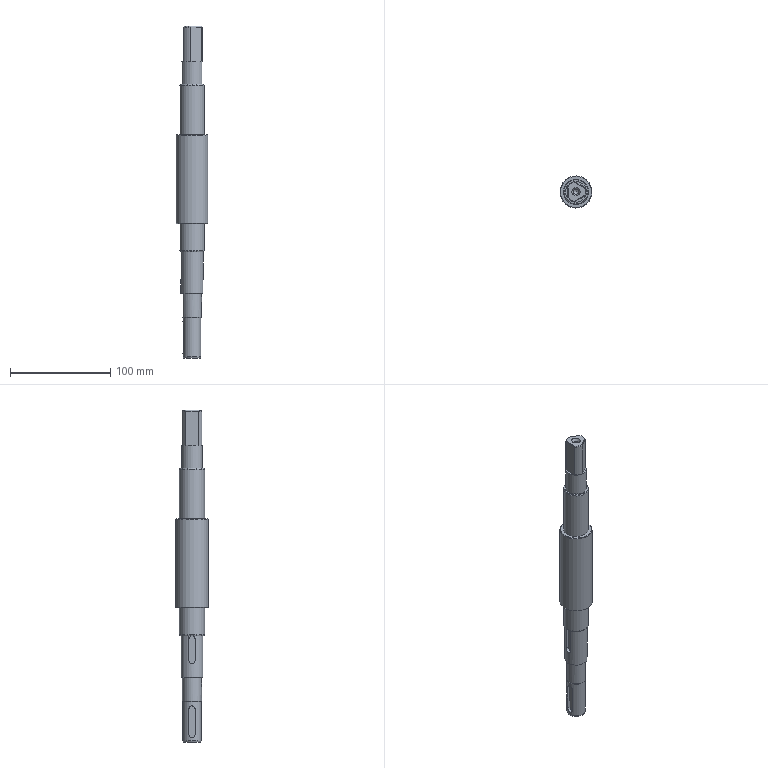NC program | NX | posted with a generic post | part box 32 x 32 x 331.3 mm
Whole program:
N10 G17 G21 G94 G90
(刀补6 , TOOL : D4)
N12 T04 M6
N14 G54
N16 G17 G0 G90 X69.382 Y0.933 B0. C0. S6685 M3
N18 G43 Z30. H4
N20 Z-2.94
N22 G94 G1 X62.644 Z-3.293 F1000.
N24 X62.507 Y0.932 Z-3.3
N26 X62.223 Y0.84 Z-3.316
N28 X61.982 Y0.664 Z-3.331
N30 X61.808 Y0.422 Z-3.347
N32 X61.718 Y0.137 Z-3.363
N34 Y-0.137 Z-3.377
N36 X61.808 Y-0.422 Z-3.393
N38 X61.982 Y-0.664 Z-3.408
N40 X62.223 Y-0.84 Z-3.424
N42 X62.507 Y-0.932 Z-3.44
N44 X62.646 Y-0.933 Z-3.447
N46 X73.552 Z-4.018
N48 G41 X73.65 Y-0.95 D4
N50 X84.656 F1650.
N52 G3 X85.599 Y0. R0.95
N54 X84.656 Y0.95 R0.95
N56 G1 X62.644
N58 G3 X61.701 Y0. R0.95
N60 X62.644 Y-0.95 R0.95
N62 G1 X73.65
N64 X78.154 Z-4.097
N66 X84.656
N68 G3 X85.599 Y0. R0.95
N70 X84.656 Y0.95 R0.95
N72 G1 X62.644
N74 G3 X61.701 Y0. R0.95
N76 X62.644 Y-0.95 R0.95
N78 G1 X73.65
N80 X78.154 Z-4.176
N82 X84.656
N84 G3 X85.599 Y0. R0.95
N86 X84.656 Y0.95 R0.95
N88 G1 X62.644
N90 G3 X61.701 Y0. R0.95
N92 X62.644 Y-0.95 R0.95
N94 G1 X73.65
N96 X78.154 Z-4.254
N98 X84.656
N100 G3 X85.599 Y0. R0.95
N102 X84.656 Y0.95 R0.95
N104 G1 X62.644
N106 G3 X61.701 Y0. R0.95
N108 X62.644 Y-0.95 R0.95
N110 G1 X73.65
N112 X78.154 Z-4.333
N114 X84.656
N116 G3 X85.599 Y0. R0.95
N118 X84.656 Y0.95 R0.95
N120 G1 X62.644
N122 G3 X61.701 Y0. R0.95
N124 X62.644 Y-0.95 R0.95
N126 G1 X73.65
N128 X78.154 Z-4.412
N130 X84.656
N132 G3 X85.599 Y0. R0.95
N134 X84.656 Y0.95 R0.95
N136 G1 X62.644
N138 G3 X61.701 Y0. R0.95
N140 X62.644 Y-0.95 R0.95
N142 G1 X73.65
N144 X78.154 Z-4.49
N146 X84.656
N148 G3 X85.599 Y0. R0.95
N150 X84.656 Y0.95 R0.95
N152 G1 X62.644
N154 G3 X61.701 Y0. R0.95
N156 X62.644 Y-0.95 R0.95
N158 G1 X73.65
N160 X78.154 Z-4.569
N162 X84.656
N164 G3 X85.599 Y0. R0.95
N166 X84.656 Y0.95 R0.95
N168 G1 X62.644
N170 G3 X61.701 Y0. R0.95
N172 X62.644 Y-0.95 R0.95
N174 G1 X73.65
N176 X78.154 Z-4.647
N178 X84.656
N180 G3 X85.599 Y0. R0.95
N182 X84.656 Y0.95 R0.95
N184 G1 X62.644
N186 G3 X61.701 Y0. R0.95
N188 X62.644 Y-0.95 R0.95
N190 G1 X73.65
N192 X78.154 Z-4.726
N194 X84.656
N196 G3 X85.599 Y0. R0.95
N198 X84.656 Y0.95 R0.95
N200 G1 X62.644
N202 G3 X61.701 Y0. R0.95
N204 X62.644 Y-0.95 R0.95
N206 G1 X73.65
N208 X78.154 Z-4.805
N210 X84.656
N212 G3 X85.599 Y0. R0.95
N214 X84.656 Y0.95 R0.95
N216 G1 X62.644
N218 G3 X61.701 Y0. R0.95
N220 X62.644 Y-0.95 R0.95
N222 G1 X73.65
N224 X78.154 Z-4.883
N226 X84.656
N228 G3 X85.599 Y0. R0.95
N230 X84.656 Y0.95 R0.95
N232 G1 X62.644
N234 G3 X61.701 Y0. R0.95
N236 X62.644 Y-0.95 R0.95
N238 G1 X73.65
N240 X78.154 Z-4.962
N242 X84.656
N244 G3 X85.599 Y0. R0.95
N246 X84.656 Y0.95 R0.95
N248 G1 X62.644
N250 G3 X61.701 Y0. R0.95
N252 X62.644 Y-0.95 R0.95
N254 G1 X73.65
N256 X78.154 Z-5.041
N258 X84.65
N260 G3 X85.6 Y0. R0.95
N262 X84.65 Y0.95 R0.95
N264 G1 X62.65
N266 G3 X61.7 Y0. R0.95
N268 X62.65 Y-0.95 R0.95
N270 G1 X73.65
N272 X78.154 Z-5.119
N274 X84.65
N276 G3 X85.6 Y0. R0.95
N278 X84.65 Y0.95 R0.95
N280 G1 X62.65
N282 G3 X61.7 Y0. R0.95
N284 X62.65 Y-0.95 R0.95
N286 G1 X73.65
N288 X78.154 Z-5.198
N290 X84.65
N292 G3 X85.6 Y0. R0.95
N294 X84.65 Y0.95 R0.95
N296 G1 X62.65
N298 G3 X61.7 Y0. R0.95
N300 X62.65 Y-0.95 R0.95
N302 G1 X73.65
N304 X78.154 Z-5.276
N306 X84.65
N308 G3 X85.6 Y0. R0.95
N310 X84.65 Y0.95 R0.95
N312 G1 X62.65
N314 G3 X61.7 Y0. R0.95
N316 X62.65 Y-0.95 R0.95
N318 G1 X73.65
N320 X78.154 Z-5.355
N322 X84.65
N324 G3 X85.6 Y0. R0.95
N326 X84.65 Y0.95 R0.95
N328 G1 X62.65
N330 G3 X61.7 Y0. R0.95
N332 X62.65 Y-0.95 R0.95
N334 G1 X73.65
N336 X78.154 Z-5.434
N338 X84.65
N340 G3 X85.6 Y0. R0.95
N342 X84.65 Y0.95 R0.95
N344 G1 X62.65
N346 G3 X61.7 Y0. R0.95
N348 X62.65 Y-0.95 R0.95
N350 G1 X73.65
N352 X78.154 Z-5.512
N354 X84.65
N356 G3 X85.6 Y0. R0.95
N358 X84.65 Y0.95 R0.95
N360 G1 X62.65
N362 G3 X61.7 Y0. R0.95
N364 X62.65 Y-0.95 R0.95
N366 G1 X73.65
N368 X78.154 Z-5.591
N370 X84.65
N372 G3 X85.6 Y0. R0.95
N374 X84.65 Y0.95 R0.95
N376 G1 X62.65
N378 G3 X61.7 Y0. R0.95
N380 X62.65 Y-0.95 R0.95
N382 G1 X73.65
N384 X78.154 Z-5.67
N386 X84.65
N388 G3 X85.6 Y0. R0.95
N390 X84.65 Y0.95 R0.95
N392 G1 X62.65
N394 G3 X61.7 Y0. R0.95
N396 X62.65 Y-0.95 R0.95
N398 G1 X73.65
N400 X78.154 Z-5.748
N402 X84.65
N404 G3 X85.6 Y0. R0.95
N406 X84.65 Y0.95 R0.95
N408 G1 X62.65
N410 G3 X61.7 Y0. R0.95
N412 X62.65 Y-0.95 R0.95
N414 G1 X73.65
N416 X78.154 Z-5.827
N418 X84.65
N420 G3 X85.6 Y0. R0.95
N422 X84.65 Y0.95 R0.95
N424 G1 X62.65
N426 G3 X61.7 Y0. R0.95
N428 X62.65 Y-0.95 R0.95
N430 G1 X73.65
N432 X78.154 Z-5.905
N434 X84.65
N436 G3 X85.6 Y0. R0.95
N438 X84.65 Y0.95 R0.95
N440 G1 X62.65
N442 G3 X61.7 Y0. R0.95
N444 X62.65 Y-0.95 R0.95
N446 G1 X73.65
N448 X78.154 Z-5.984
N450 X84.65
N452 G3 X85.6 Y0. R0.95
N454 X84.65 Y0.95 R0.95
N456 G1 X62.65
N458 G3 X61.7 Y0. R0.95
N460 X62.65 Y-0.95 R0.95
N462 G1 X73.65
N464 X78.154 Z-6.063
N466 X84.65
N468 G3 X85.6 Y0. R0.95
N470 X84.65 Y0.95 R0.95
N472 G1 X62.65
N474 G3 X61.7 Y0. R0.95
N476 X62.65 Y-0.95 R0.95
N478 G1 X73.65
N480 X78.154 Z-6.141
N482 X84.65
N484 G3 X85.6 Y0. R0.95
N486 X84.65 Y0.95 R0.95
N488 G1 X62.65
N490 G3 X61.7 Y0. R0.95
N492 X62.65 Y-0.95 R0.95
N494 G1 X73.65
N496 X78.154 Z-6.22
N498 X84.65
N500 G3 X85.6 Y0. R0.95
N502 X84.65 Y0.95 R0.95
N504 G1 X62.65
N506 G3 X61.7 Y0. R0.95
N508 X62.65 Y-0.95 R0.95
N510 G1 X73.65
N512 X78.154 Z-6.299
N514 X84.65
N516 G3 X85.6 Y0. R0.95
N518 X84.65 Y0.95 R0.95
N520 G1 X62.65
N522 G3 X61.7 Y0. R0.95
N524 X62.65 Y-0.95 R0.95
N526 G1 X73.65
N528 X78.154 Z-6.377
N530 X84.65
N532 G3 X85.6 Y0. R0.95
N534 X84.65 Y0.95 R0.95
N536 G1 X62.65
N538 G3 X61.7 Y0. R0.95
N540 X62.65 Y-0.95 R0.95
N542 G1 X73.65
N544 X78.154 Z-6.456
N546 X84.65
N548 G3 X85.6 Y0. R0.95
N550 X84.65 Y0.95 R0.95
N552 G1 X62.65
N554 G3 X61.7 Y0. R0.95
N556 X62.65 Y-0.95 R0.95
N558 G1 X73.65
N560 X78.154 Z-6.534
N562 X84.65
N564 G3 X85.6 Y0. R0.95
N566 X84.65 Y0.95 R0.95
N568 G1 X62.65
N570 G3 X61.7 Y0. R0.95
N572 X62.65 Y-0.95 R0.95
N574 G1 X73.65
N576 X78.154 Z-6.613
N578 X84.65
N580 G3 X85.6 Y0. R0.95
N582 X84.65 Y0.95 R0.95
N584 G1 X62.65
N586 G3 X61.7 Y0. R0.95
N588 X62.65 Y-0.95 R0.95
N590 G1 X73.65
N592 X78.154 Z-6.692
N594 X84.65
N596 G3 X85.6 Y0. R0.95
N598 X84.65 Y0.95 R0.95
N600 G1 X62.65
N602 G3 X61.7 Y0. R0.95
N604 X62.65 Y-0.95 R0.95
N606 G1 X73.65
N608 X78.154 Z-6.77
N610 X84.65
N612 G3 X85.6 Y0. R0.95
N614 X84.65 Y0.95 R0.95
N616 G1 X62.65
N618 G3 X61.7 Y0. R0.95
N620 X62.65 Y-0.95 R0.95
N622 G1 X73.65
N624 X78.154 Z-6.849
N626 X84.65
N628 G3 X85.6 Y0. R0.95
N630 X84.65 Y0.95 R0.95
N632 G1 X62.65
N634 G3 X61.7 Y0. R0.95
N636 X62.65 Y-0.95 R0.95
N638 G1 X73.65
N640 X78.154 Z-6.928
N642 X84.65
N644 G3 X85.6 Y0. R0.95
N646 X84.65 Y0.95 R0.95
N648 G1 X62.65
N650 G3 X61.7 Y0. R0.95
N652 X62.65 Y-0.95 R0.95
N654 G1 X73.65
N656 X78.154 Z-7.006
N658 X84.65
N660 G3 X85.6 Y0. R0.95
N662 X84.65 Y0.95 R0.95
N664 G1 X62.65
N666 G3 X61.7 Y0. R0.95
N668 X62.65 Y-0.95 R0.95
N670 G1 X73.65
N672 X78.154 Z-7.085
N674 X84.65
N676 G3 X85.6 Y0. R0.95
N678 X84.65 Y0.95 R0.95
N680 G1 X62.65
N682 G3 X61.7 Y0. R0.95
N684 X62.65 Y-0.95 R0.95
N686 G1 X73.65
N688 X78.154 Z-7.163
N690 X84.65
N692 G3 X85.6 Y0. R0.95
N694 X84.65 Y0.95 R0.95
N696 G1 X62.65
N698 G3 X61.7 Y0. R0.95
N700 X62.65 Y-0.95 R0.95
N702 G1 X73.65
N704 X78.154 Z-7.242
N706 X84.65
N708 G3 X85.6 Y0. R0.95
N710 X84.65 Y0.95 R0.95
N712 G1 X62.65
N714 G3 X61.7 Y0. R0.95
N716 X62.65 Y-0.95 R0.95
N718 G1 X73.65
N720 X78.154 Z-7.321
N722 X84.65
N724 G3 X85.6 Y0. R0.95
N726 X84.65 Y0.95 R0.95
N728 G1 X62.65
N730 G3 X61.7 Y0. R0.95
N732 X62.65 Y-0.95 R0.95
N734 G1 X73.65
N736 X78.154 Z-7.399
N738 X84.65
N740 G3 X85.6 Y0. R0.95
N742 X84.65 Y0.95 R0.95
N744 G1 X62.65
N746 G3 X61.7 Y0. R0.95
N748 X62.65 Y-0.95 R0.95
N750 G1 X73.65
N752 X78.154 Z-7.478
N754 X84.65
N756 G3 X85.6 Y0. R0.95
N758 X84.65 Y0.95 R0.95
N760 G1 X62.65
N762 G3 X61.7 Y0. R0.95
N764 X62.65 Y-0.95 R0.95
N766 G1 X73.65
N768 X78.154 Z-7.557
N770 X84.65
N772 G3 X85.6 Y0. R0.95
N774 X84.65 Y0.95 R0.95
N776 G1 X62.65
N778 G3 X61.7 Y0. R0.95
N780 X62.65 Y-0.95 R0.95
N782 G1 X73.65
N784 X78.154 Z-7.635
N786 X84.65
N788 G3 X85.6 Y0. R0.95
N790 X84.65 Y0.95 R0.95
N792 G1 X62.65
N794 G3 X61.7 Y0. R0.95
N796 X62.65 Y-0.95 R0.95
N798 G1 X73.65
N800 X78.154 Z-7.714
N802 X84.65
N804 G3 X85.6 Y0. R0.95
N806 X84.65 Y0.95 R0.95
N808 G1 X62.65
N810 G3 X61.7 Y0. R0.95
N812 X62.65 Y-0.95 R0.95
N814 G1 X73.65
N816 X78.154 Z-7.792
N818 X84.65
N820 G3 X85.6 Y0. R0.95
N822 X84.65 Y0.95 R0.95
N824 G1 X62.65
N826 G3 X61.7 Y0. R0.95
N828 X62.65 Y-0.95 R0.95
N830 G1 X73.65
N832 X78.154 Z-7.871
N834 X84.65
N836 G3 X85.6 Y0. R0.95
N838 X84.65 Y0.95 R0.95
N840 G1 X62.65
N842 G3 X61.7 Y0. R0.95
N844 X62.65 Y-0.95 R0.95
N846 G1 X73.65
N848 X78.154 Z-7.95
N850 X84.65
N852 G3 X85.6 Y0. R0.95
N854 X84.65 Y0.95 R0.95
N856 G1 X62.65
N858 G3 X61.7 Y0. R0.95
N860 X62.65 Y-0.95 R0.95
N862 G1 X73.65
N864 X78.154 Z-8.028
N866 X84.65
N868 G3 X85.6 Y0. R0.95
N870 X84.65 Y0.95 R0.95
N872 G1 X62.65
N874 G3 X61.7 Y0. R0.95
N876 X62.65 Y-0.95 R0.95
N878 G1 X73.65
N880 X78.154 Z-8.107
N882 X84.65
N884 G3 X85.6 Y0. R0.95
N886 X84.65 Y0.95 R0.95
N888 G1 X62.65
N890 G3 X61.7 Y0. R0.95
N892 X62.65 Y-0.95 R0.95
N894 G1 X73.65
N896 X78.154 Z-8.186
N898 X84.65
N900 G3 X85.6 Y0. R0.95
N902 X84.65 Y0.95 R0.95
N904 G1 X62.65
N906 G3 X61.7 Y0. R0.95
N908 X62.65 Y-0.95 R0.95
N910 G1 X73.65
N912 X78.154 Z-8.264
N914 X84.65
N916 G3 X85.6 Y0. R0.95
N918 X84.65 Y0.95 R0.95
N920 G1 X62.65
N922 G3 X61.7 Y0. R0.95
N924 X62.65 Y-0.95 R0.95
N926 G1 X73.65
N928 X78.154 Z-8.343
N930 X84.65
N932 G3 X85.6 Y0. R0.95
N934 X84.65 Y0.95 R0.95
N936 G1 X62.65
N938 G3 X61.7 Y0. R0.95
N940 X62.65 Y-0.95 R0.95
N942 G1 X73.65
N944 X78.154 Z-8.421
N946 X84.65
N948 G3 X85.6 Y0. R0.95
N950 X84.65 Y0.95 R0.95
N952 G1 X62.65
N954 G3 X61.7 Y0. R0.95
N956 X62.65 Y-0.95 R0.95
N958 G1 X73.65
N960 X78.154 Z-8.5
N962 X84.65
N964 G3 X85.6 Y0. R0.95
N966 X84.65 Y0.95 R0.95
N968 G1 X62.65
N970 G3 X61.7 Y0. R0.95
N972 X62.65 Y-0.95 R0.95
N974 G1 X78.154
N976 G40
N978 X78.253 Y-0.933
N980 Z-7.5
N982 G0 Z30.
(刀补6_COPY , TOOL : D4)
N984 X137.381 Y0.933
N986 Z-5.884
N988 G1 X132.644 Z-6.133 F1000.
N990 X132.507 Y0.932 Z-6.14
N992 X132.223 Y0.84 Z-6.156
N994 X131.982 Y0.664 Z-6.171
N996 X131.808 Y0.422 Z-6.187
N998 X131.718 Y0.137 Z-6.203
N1000 Y-0.137 Z-6.217
N1002 X131.808 Y-0.422 Z-6.233
N1004 X131.982 Y-0.664 Z-6.248
N1006 X132.223 Y-0.84 Z-6.264
N1008 X132.507 Y-0.932 Z-6.279
N1010 X132.646 Y-0.933 Z-6.287
N1012 X145.552 Z-6.963
N1014 G41 X145.65 Y-0.95
N1016 X158.656 F1650.
N1018 G3 X159.599 Y0. R0.95
N1020 X158.656 Y0.95 R0.95
N1022 G1 X132.644
N1024 G3 X131.701 Y0. R0.95
N1026 X132.644 Y-0.95 R0.95
N1028 G1 X145.65
N1030 X150.153 Z-7.042
N1032 X158.65
N1034 G3 X159.6 Y0. R0.95
N1036 X158.65 Y0.95 R0.95
N1038 G1 X132.65
N1040 G3 X131.7 Y0. R0.95
N1042 X132.65 Y-0.95 R0.95
N1044 G1 X145.65
N1046 X150.153 Z-7.12
N1048 X158.65
N1050 G3 X159.6 Y0. R0.95
N1052 X158.65 Y0.95 R0.95
N1054 G1 X132.65
N1056 G3 X131.7 Y0. R0.95
N1058 X132.65 Y-0.95 R0.95
N1060 G1 X145.65
N1062 X150.153 Z-7.199
N1064 X158.65
N1066 G3 X159.6 Y0. R0.95
N1068 X158.65 Y0.95 R0.95
N1070 G1 X132.65
N1072 G3 X131.7 Y0. R0.95
N1074 X132.65 Y-0.95 R0.95
N1076 G1 X145.65
N1078 X150.153 Z-7.277
N1080 X158.65
N1082 G3 X159.6 Y0. R0.95
N1084 X158.65 Y0.95 R0.95
N1086 G1 X132.65
N1088 G3 X131.7 Y0. R0.95
N1090 X132.65 Y-0.95 R0.95
N1092 G1 X145.65
N1094 X150.153 Z-7.356
N1096 X158.65
N1098 G3 X159.6 Y0. R0.95
N1100 X158.65 Y0.95 R0.95
N1102 G1 X132.65
N1104 G3 X131.7 Y0. R0.95
N1106 X132.65 Y-0.95 R0.95
N1108 G1 X145.65
N1110 X150.153 Z-7.435
N1112 X158.65
N1114 G3 X159.6 Y0. R0.95
N1116 X158.65 Y0.95 R0.95
N1118 G1 X132.65
N1120 G3 X131.7 Y0. R0.95
N1122 X132.65 Y-0.95 R0.95
N1124 G1 X145.65
N1126 X150.153 Z-7.513
N1128 X158.65
N1130 G3 X159.6 Y0. R0.95
N1132 X158.65 Y0.95 R0.95
N1134 G1 X132.65
N1136 G3 X131.7 Y0. R0.95
N1138 X132.65 Y-0.95 R0.95
N1140 G1 X145.65
N1142 X150.153 Z-7.592
N1144 X158.65
N1146 G3 X159.6 Y0. R0.95
N1148 X158.65 Y0.95 R0.95
N1150 G1 X132.65
N1152 G3 X131.7 Y0. R0.95
N1154 X132.65 Y-0.95 R0.95
N1156 G1 X145.65
N1158 X150.153 Z-7.67
N1160 X158.65
N1162 G3 X159.6 Y0. R0.95
N1164 X158.65 Y0.95 R0.95
N1166 G1 X132.65
N1168 G3 X131.7 Y0. R0.95
N1170 X132.65 Y-0.95 R0.95
N1172 G1 X145.65
N1174 X150.153 Z-7.749
N1176 X158.65
N1178 G3 X159.6 Y0. R0.95
N1180 X158.65 Y0.95 R0.95
N1182 G1 X132.65
N1184 G3 X131.7 Y0. R0.95
N1186 X132.65 Y-0.95 R0.95
N1188 G1 X145.65
N1190 X150.153 Z-7.828
N1192 X158.65
N1194 G3 X159.6 Y0. R0.95
N1196 X158.65 Y0.95 R0.95
N1198 G1 X132.65
N1200 G3 X131.7 Y0. R0.95
N1202 X132.65 Y-0.95 R0.95
N1204 G1 X145.65
N1206 X150.153 Z-7.906
N1208 X158.65
N1210 G3 X159.6 Y0. R0.95
N1212 X158.65 Y0.95 R0.95
N1214 G1 X132.65
N1216 G3 X131.7 Y0. R0.95
N1218 X132.65 Y-0.95 R0.95
N1220 G1 X145.65
N1222 X150.153 Z-7.985
N1224 X158.65
N1226 G3 X159.6 Y0. R0.95
N1228 X158.65 Y0.95 R0.95
N1230 G1 X132.65
N1232 G3 X131.7 Y0. R0.95
N1234 X132.65 Y-0.95 R0.95
N1236 G1 X145.65
N1238 X150.153 Z-8.063
N1240 X158.65
N1242 G3 X159.6 Y0. R0.95
N1244 X158.65 Y0.95 R0.95
N1246 G1 X132.65
N1248 G3 X131.7 Y0. R0.95
N1250 X132.65 Y-0.95 R0.95
N1252 G1 X145.65
N1254 X150.153 Z-8.142
N1256 X158.65
N1258 G3 X159.6 Y0. R0.95
N1260 X158.65 Y0.95 R0.95
N1262 G1 X132.65
N1264 G3 X131.7 Y0. R0.95
N1266 X132.65 Y-0.95 R0.95
N1268 G1 X145.65
N1270 X150.153 Z-8.221
N1272 X158.65
N1274 G3 X159.6 Y0. R0.95
N1276 X158.65 Y0.95 R0.95
N1278 G1 X132.65
N1280 G3 X131.7 Y0. R0.95
N1282 X132.65 Y-0.95 R0.95
N1284 G1 X145.65
N1286 X150.153 Z-8.299
N1288 X158.65
N1290 G3 X159.6 Y0. R0.95
N1292 X158.65 Y0.95 R0.95
N1294 G1 X132.65
N1296 G3 X131.7 Y0. R0.95
N1298 X132.65 Y-0.95 R0.95
N1300 G1 X145.65
N1302 X150.153 Z-8.378
N1304 X158.65
N1306 G3 X159.6 Y0. R0.95
N1308 X158.65 Y0.95 R0.95
N1310 G1 X132.65
N1312 G3 X131.7 Y0. R0.95
N1314 X132.65 Y-0.95 R0.95
N1316 G1 X145.65
N1318 X150.153 Z-8.456
N1320 X158.65
N1322 G3 X159.6 Y0. R0.95
N1324 X158.65 Y0.95 R0.95
N1326 G1 X132.65
N1328 G3 X131.7 Y0. R0.95
N1330 X132.65 Y-0.95 R0.95
N1332 G1 X145.65
N1334 X150.153 Z-8.535
N1336 X158.65
N1338 G3 X159.6 Y0. R0.95
N1340 X158.65 Y0.95 R0.95
N1342 G1 X132.65
N1344 G3 X131.7 Y0. R0.95
N1346 X132.65 Y-0.95 R0.95
N1348 G1 X145.65
N1350 X150.153 Z-8.614
N1352 X158.65
N1354 G3 X159.6 Y0. R0.95
N1356 X158.65 Y0.95 R0.95
N1358 G1 X132.65
N1360 G3 X131.7 Y0. R0.95
N1362 X132.65 Y-0.95 R0.95
N1364 G1 X145.65
N1366 X150.153 Z-8.692
N1368 X158.65
N1370 G3 X159.6 Y0. R0.95
N1372 X158.65 Y0.95 R0.95
N1374 G1 X132.65
N1376 G3 X131.7 Y0. R0.95
N1378 X132.65 Y-0.95 R0.95
N1380 G1 X145.65
N1382 X150.153 Z-8.771
N1384 X158.65
N1386 G3 X159.6 Y0. R0.95
N1388 X158.65 Y0.95 R0.95
N1390 G1 X132.65
N1392 G3 X131.7 Y0. R0.95
N1394 X132.65 Y-0.95 R0.95
N1396 G1 X145.65
N1398 X150.153 Z-8.849
N1400 X158.65
N1402 G3 X159.6 Y0. R0.95
N1404 X158.65 Y0.95 R0.95
N1406 G1 X132.65
N1408 G3 X131.7 Y0. R0.95
N1410 X132.65 Y-0.95 R0.95
N1412 G1 X145.65
N1414 X150.153 Z-8.928
N1416 X158.65
N1418 G3 X159.6 Y0. R0.95
N1420 X158.65 Y0.95 R0.95
N1422 G1 X132.65
N1424 G3 X131.7 Y0. R0.95
N1426 X132.65 Y-0.95 R0.95
N1428 G1 X145.65
N1430 X150.153 Z-9.007
N1432 X158.65
N1434 G3 X159.6 Y0. R0.95
N1436 X158.65 Y0.95 R0.95
N1438 G1 X132.65
N1440 G3 X131.7 Y0. R0.95
N1442 X132.65 Y-0.95 R0.95
N1444 G1 X145.65
N1446 X150.153 Z-9.085
N1448 X158.65
N1450 G3 X159.6 Y0. R0.95
N1452 X158.65 Y0.95 R0.95
N1454 G1 X132.65
N1456 G3 X131.7 Y0. R0.95
N1458 X132.65 Y-0.95 R0.95
N1460 G1 X145.65
N1462 X150.153 Z-9.164
N1464 X158.65
N1466 G3 X159.6 Y0. R0.95
N1468 X158.65 Y0.95 R0.95
N1470 G1 X132.65
N1472 G3 X131.7 Y0. R0.95
N1474 X132.65 Y-0.95 R0.95
N1476 G1 X145.65
N1478 X150.153 Z-9.242
N1480 X158.65
N1482 G3 X159.6 Y0. R0.95
N1484 X158.65 Y0.95 R0.95
N1486 G1 X132.65
N1488 G3 X131.7 Y0. R0.95
N1490 X132.65 Y-0.95 R0.95
N1492 G1 X145.65
N1494 X150.153 Z-9.321
N1496 X158.65
N1498 G3 X159.6 Y0. R0.95
N1500 X158.65 Y0.95 R0.95
N1502 G1 X132.65
N1504 G3 X131.7 Y0. R0.95
N1506 X132.65 Y-0.95 R0.95
N1508 G1 X145.65
N1510 X150.153 Z-9.4
N1512 X158.65
N1514 G3 X159.6 Y0. R0.95
N1516 X158.65 Y0.95 R0.95
N1518 G1 X132.65
N1520 G3 X131.7 Y0. R0.95
N1522 X132.65 Y-0.95 R0.95
N1524 G1 X145.65
N1526 X150.153 Z-9.478
N1528 X158.65
N1530 G3 X159.6 Y0. R0.95
N1532 X158.65 Y0.95 R0.95
N1534 G1 X132.65
N1536 G3 X131.7 Y0. R0.95
N1538 X132.65 Y-0.95 R0.95
N1540 G1 X145.65
N1542 X150.153 Z-9.557
N1544 X158.65
N1546 G3 X159.6 Y0. R0.95
N1548 X158.65 Y0.95 R0.95
N1550 G1 X132.65
N1552 G3 X131.7 Y0. R0.95
N1554 X132.65 Y-0.95 R0.95
N1556 G1 X145.65
N1558 X150.153 Z-9.635
N1560 X158.65
N1562 G3 X159.6 Y0. R0.95
N1564 X158.65 Y0.95 R0.95
N1566 G1 X132.65
N1568 G3 X131.7 Y0. R0.95
N1570 X132.65 Y-0.95 R0.95
N1572 G1 X145.65
N1574 X150.153 Z-9.714
N1576 X158.65
N1578 G3 X159.6 Y0. R0.95
N1580 X158.65 Y0.95 R0.95
N1582 G1 X132.65
N1584 G3 X131.7 Y0. R0.95
N1586 X132.65 Y-0.95 R0.95
N1588 G1 X145.65
N1590 X150.153 Z-9.793
N1592 X158.65
N1594 G3 X159.6 Y0. R0.95
N1596 X158.65 Y0.95 R0.95
N1598 G1 X132.65
N1600 G3 X131.7 Y0. R0.95
N1602 X132.65 Y-0.95 R0.95
N1604 G1 X145.65
N1606 X150.153 Z-9.871
N1608 X158.65
N1610 G3 X159.6 Y0. R0.95
N1612 X158.65 Y0.95 R0.95
N1614 G1 X132.65
N1616 G3 X131.7 Y0. R0.95
N1618 X132.65 Y-0.95 R0.95
N1620 G1 X145.65
N1622 X150.153 Z-9.95
N1624 X158.65
N1626 G3 X159.6 Y0. R0.95
N1628 X158.65 Y0.95 R0.95
N1630 G1 X132.65
N1632 G3 X131.7 Y0. R0.95
N1634 X132.65 Y-0.95 R0.95
N1636 G1 X145.65
N1638 X150.153 Z-10.028
N1640 X158.65
N1642 G3 X159.6 Y0. R0.95
N1644 X158.65 Y0.95 R0.95
N1646 G1 X132.65
N1648 G3 X131.7 Y0. R0.95
N1650 X132.65 Y-0.95 R0.95
N1652 G1 X145.65
N1654 X150.153 Z-10.107
N1656 X158.65
N1658 G3 X159.6 Y0. R0.95
N1660 X158.65 Y0.95 R0.95
N1662 G1 X132.65
N1664 G3 X131.7 Y0. R0.95
N1666 X132.65 Y-0.95 R0.95
N1668 G1 X145.65
N1670 X150.153 Z-10.186
N1672 X158.65
N1674 G3 X159.6 Y0. R0.95
N1676 X158.65 Y0.95 R0.95
N1678 G1 X132.65
N1680 G3 X131.7 Y0. R0.95
N1682 X132.65 Y-0.95 R0.95
N1684 G1 X145.65
N1686 X150.153 Z-10.264
N1688 X158.65
N1690 G3 X159.6 Y0. R0.95
N1692 X158.65 Y0.95 R0.95
N1694 G1 X132.65
N1696 G3 X131.7 Y0. R0.95
N1698 X132.65 Y-0.95 R0.95
N1700 G1 X145.65
N1702 X150.153 Z-10.343
N1704 X158.65
N1706 G3 X159.6 Y0. R0.95
N1708 X158.65 Y0.95 R0.95
N1710 G1 X132.65
N1712 G3 X131.7 Y0. R0.95
N1714 X132.65 Y-0.95 R0.95
N1716 G1 X145.65
N1718 X150.153 Z-10.421
N1720 X158.65
N1722 G3 X159.6 Y0. R0.95
N1724 X158.65 Y0.95 R0.95
N1726 G1 X132.65
N1728 G3 X131.7 Y0. R0.95
N1730 X132.65 Y-0.95 R0.95
N1732 G1 X145.65
N1734 X150.153 Z-10.5
N1736 X158.65
N1738 G3 X159.6 Y0. R0.95
N1740 X158.65 Y0.95 R0.95
N1742 G1 X132.65
N1744 G3 X131.7 Y0. R0.95
N1746 X132.65 Y-0.95 R0.95
N1748 G1 X150.153
N1750 G40
N1752 X150.251 Y-0.933
N1754 Z-9.5
N1756 G0 Z30.
N1758 M5
N1760 M2